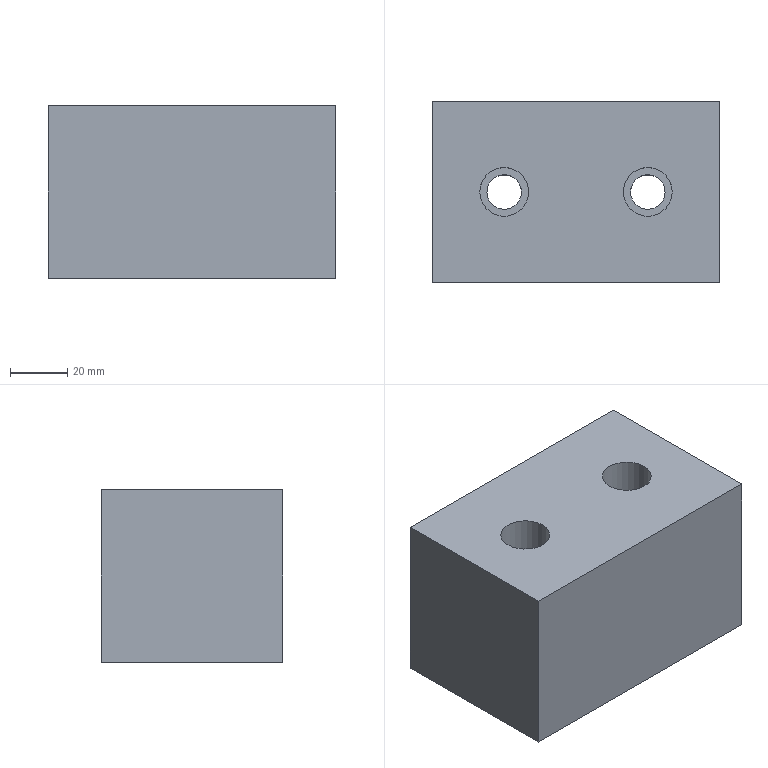Part | NX | features solid 2 | 1 solid | 12 faces | box 100 x 63 x 60 mm | volume 355318 mm3 | plane 8 | cylinder 4 | commonest cylinder face diameters 12 x2 17 x2
STEP:
#1=CARTESIAN_POINT('',(1065.,781.5,-55.));
#2=VERTEX_POINT('',#1);
#3=CARTESIAN_POINT('',(1065.,781.5,5.));
#4=VERTEX_POINT('',#3);
#5=CARTESIAN_POINT('',(1065.,781.5,-55.));
#6=DIRECTION('',(0.,0.,-1.));
#7=VECTOR('',#6,1000.);
#8=LINE('',#5,#7);
#9=EDGE_CURVE('',#2,#4,#8,.F.);
#10=ORIENTED_EDGE('',*,*,#9,.T.);
#11=CARTESIAN_POINT('',(1165.,781.5,5.));
#12=VERTEX_POINT('',#11);
#13=CARTESIAN_POINT('',(1065.,781.5,5.));
#14=DIRECTION('',(1.,0.,0.));
#15=VECTOR('',#14,1000.);
#16=LINE('',#13,#15);
#17=EDGE_CURVE('',#4,#12,#16,.T.);
#18=ORIENTED_EDGE('',*,*,#17,.T.);
#19=CARTESIAN_POINT('',(1165.,781.5,-55.));
#20=VERTEX_POINT('',#19);
#21=CARTESIAN_POINT('',(1165.,781.5,-55.));
#22=DIRECTION('',(0.,0.,1.));
#23=VECTOR('',#22,1000.);
#24=LINE('',#21,#23);
#25=EDGE_CURVE('',#20,#12,#24,.T.);
#26=ORIENTED_EDGE('',*,*,#25,.F.);
#27=CARTESIAN_POINT('',(1065.,781.5,-55.));
#28=DIRECTION('',(1.,0.,0.));
#29=VECTOR('',#28,1000.);
#30=LINE('',#27,#29);
#31=EDGE_CURVE('',#2,#20,#30,.T.);
#32=ORIENTED_EDGE('',*,*,#31,.F.);
#33=EDGE_LOOP('',(#10,#18,#26,#32));
#34=FACE_BOUND('',#33,.T.);
#35=CARTESIAN_POINT('',(1065.,781.5,-55.));
#36=DIRECTION('',(0.,1.,0.));
#37=DIRECTION('',(1.,0.,0.));
#38=AXIS2_PLACEMENT_3D('',#35,#36,#37);
#39=PLANE('',#38);
#40=ADVANCED_FACE('',(#34),#39,.T.);
#41=ORIENTED_EDGE('',*,*,#25,.T.);
#42=CARTESIAN_POINT('',(1165.,718.5,5.));
#43=VERTEX_POINT('',#42);
#44=CARTESIAN_POINT('',(1165.,780.,5.));
#45=DIRECTION('',(0.,-1.,0.));
#46=VECTOR('',#45,1000.);
#47=LINE('',#44,#46);
#48=EDGE_CURVE('',#12,#43,#47,.T.);
#49=ORIENTED_EDGE('',*,*,#48,.T.);
#50=CARTESIAN_POINT('',(1165.,718.5,-55.));
#51=VERTEX_POINT('',#50);
#52=CARTESIAN_POINT('',(1165.,718.5,-55.));
#53=DIRECTION('',(0.,0.,-1.));
#54=VECTOR('',#53,1000.);
#55=LINE('',#52,#54);
#56=EDGE_CURVE('',#51,#43,#55,.F.);
#57=ORIENTED_EDGE('',*,*,#56,.F.);
#58=CARTESIAN_POINT('',(1165.,780.,-55.));
#59=DIRECTION('',(0.,-1.,0.));
#60=VECTOR('',#59,1000.);
#61=LINE('',#58,#60);
#62=EDGE_CURVE('',#20,#51,#61,.T.);
#63=ORIENTED_EDGE('',*,*,#62,.F.);
#64=EDGE_LOOP('',(#41,#49,#57,#63));
#65=FACE_BOUND('',#64,.T.);
#66=CARTESIAN_POINT('',(1165.,780.,-55.));
#67=DIRECTION('',(1.,0.,0.));
#68=DIRECTION('',(0.,-1.,0.));
#69=AXIS2_PLACEMENT_3D('',#66,#67,#68);
#70=PLANE('',#69);
#71=ADVANCED_FACE('',(#65),#70,.T.);
#72=ORIENTED_EDGE('',*,*,#56,.T.);
#73=CARTESIAN_POINT('',(1065.,718.5,5.));
#74=VERTEX_POINT('',#73);
#75=CARTESIAN_POINT('',(1065.,718.5,5.));
#76=DIRECTION('',(-1.,0.,0.));
#77=VECTOR('',#76,1000.);
#78=LINE('',#75,#77);
#79=EDGE_CURVE('',#74,#43,#78,.F.);
#80=ORIENTED_EDGE('',*,*,#79,.F.);
#81=CARTESIAN_POINT('',(1065.,718.5,-55.));
#82=VERTEX_POINT('',#81);
#83=CARTESIAN_POINT('',(1065.,718.5,-55.));
#84=DIRECTION('',(0.,0.,1.));
#85=VECTOR('',#84,1000.);
#86=LINE('',#83,#85);
#87=EDGE_CURVE('',#82,#74,#86,.T.);
#88=ORIENTED_EDGE('',*,*,#87,.F.);
#89=CARTESIAN_POINT('',(1065.,718.5,-55.));
#90=DIRECTION('',(-1.,0.,0.));
#91=VECTOR('',#90,1000.);
#92=LINE('',#89,#91);
#93=EDGE_CURVE('',#82,#51,#92,.F.);
#94=ORIENTED_EDGE('',*,*,#93,.T.);
#95=EDGE_LOOP('',(#72,#80,#88,#94));
#96=FACE_BOUND('',#95,.T.);
#97=CARTESIAN_POINT('',(1065.,718.5,-55.));
#98=DIRECTION('',(0.,1.,0.));
#99=DIRECTION('',(1.,0.,0.));
#100=AXIS2_PLACEMENT_3D('',#97,#98,#99);
#101=PLANE('',#100);
#102=ADVANCED_FACE('',(#96),#101,.F.);
#103=CARTESIAN_POINT('',(1065.,780.,-55.));
#104=DIRECTION('',(0.,-1.,0.));
#105=VECTOR('',#104,1000.);
#106=LINE('',#103,#105);
#107=EDGE_CURVE('',#2,#82,#106,.T.);
#108=ORIENTED_EDGE('',*,*,#107,.T.);
#109=ORIENTED_EDGE('',*,*,#87,.T.);
#110=CARTESIAN_POINT('',(1065.,780.,5.));
#111=DIRECTION('',(0.,1.,0.));
#112=VECTOR('',#111,1000.);
#113=LINE('',#110,#112);
#114=EDGE_CURVE('',#4,#74,#113,.F.);
#115=ORIENTED_EDGE('',*,*,#114,.F.);
#116=ORIENTED_EDGE('',*,*,#9,.F.);
#117=EDGE_LOOP('',(#108,#109,#115,#116));
#118=FACE_BOUND('',#117,.T.);
#119=CARTESIAN_POINT('',(1065.,780.,-55.));
#120=DIRECTION('',(1.,0.,0.));
#121=DIRECTION('',(0.,-1.,0.));
#122=AXIS2_PLACEMENT_3D('',#119,#120,#121);
#123=PLANE('',#122);
#124=ADVANCED_FACE('',(#118),#123,.F.);
#125=CARTESIAN_POINT('',(1131.5,750.,5.));
#126=VERTEX_POINT('',#125);
#127=CARTESIAN_POINT('',(1140.,750.,5.));
#128=DIRECTION('',(0.,0.,1.));
#129=DIRECTION('',(-1.,0.,0.));
#130=AXIS2_PLACEMENT_3D('',#127,#128,#129);
#131=CIRCLE('',#130,8.5);
#132=EDGE_CURVE('',#126,#126,#131,.T.);
#133=ORIENTED_EDGE('',*,*,#132,.F.);
#134=EDGE_LOOP('',(#133));
#135=FACE_BOUND('',#134,.T.);
#136=CARTESIAN_POINT('',(1081.5,750.,5.));
#137=VERTEX_POINT('',#136);
#138=CARTESIAN_POINT('',(1090.,750.,5.));
#139=DIRECTION('',(0.,0.,1.));
#140=DIRECTION('',(-1.,0.,0.));
#141=AXIS2_PLACEMENT_3D('',#138,#139,#140);
#142=CIRCLE('',#141,8.5);
#143=EDGE_CURVE('',#137,#137,#142,.T.);
#144=ORIENTED_EDGE('',*,*,#143,.F.);
#145=EDGE_LOOP('',(#144));
#146=FACE_BOUND('',#145,.T.);
#147=ORIENTED_EDGE('',*,*,#79,.T.);
#148=ORIENTED_EDGE('',*,*,#48,.F.);
#149=ORIENTED_EDGE('',*,*,#17,.F.);
#150=ORIENTED_EDGE('',*,*,#114,.T.);
#151=EDGE_LOOP('',(#147,#148,#149,#150));
#152=FACE_BOUND('',#151,.T.);
#153=CARTESIAN_POINT('',(1065.,780.,5.));
#154=DIRECTION('',(0.,0.,1.));
#155=DIRECTION('',(1.,0.,0.));
#156=AXIS2_PLACEMENT_3D('',#153,#154,#155);
#157=PLANE('',#156);
#158=ADVANCED_FACE('',(#135,#146,#152),#157,.T.);
#159=CARTESIAN_POINT('',(1146.,750.,-55.));
#160=VERTEX_POINT('',#159);
#161=CARTESIAN_POINT('',(1140.,750.,-55.));
#162=DIRECTION('',(0.,0.,-1.));
#163=DIRECTION('',(1.,0.,0.));
#164=AXIS2_PLACEMENT_3D('',#161,#162,#163);
#165=CIRCLE('',#164,6.);
#166=EDGE_CURVE('',#160,#160,#165,.T.);
#167=ORIENTED_EDGE('',*,*,#166,.F.);
#168=EDGE_LOOP('',(#167));
#169=FACE_BOUND('',#168,.T.);
#170=CARTESIAN_POINT('',(1096.,750.,-55.));
#171=VERTEX_POINT('',#170);
#172=CARTESIAN_POINT('',(1090.,750.,-55.));
#173=DIRECTION('',(0.,0.,-1.));
#174=DIRECTION('',(1.,0.,0.));
#175=AXIS2_PLACEMENT_3D('',#172,#173,#174);
#176=CIRCLE('',#175,6.);
#177=EDGE_CURVE('',#171,#171,#176,.T.);
#178=ORIENTED_EDGE('',*,*,#177,.F.);
#179=EDGE_LOOP('',(#178));
#180=FACE_BOUND('',#179,.T.);
#181=ORIENTED_EDGE('',*,*,#93,.F.);
#182=ORIENTED_EDGE('',*,*,#107,.F.);
#183=ORIENTED_EDGE('',*,*,#31,.T.);
#184=ORIENTED_EDGE('',*,*,#62,.T.);
#185=EDGE_LOOP('',(#181,#182,#183,#184));
#186=FACE_BOUND('',#185,.T.);
#187=CARTESIAN_POINT('',(1065.,780.,-55.));
#188=DIRECTION('',(0.,0.,1.));
#189=DIRECTION('',(1.,0.,0.));
#190=AXIS2_PLACEMENT_3D('',#187,#188,#189);
#191=PLANE('',#190);
#192=ADVANCED_FACE('',(#169,#180,#186),#191,.F.);
#193=CARTESIAN_POINT('',(1084.,750.,-35.));
#194=VERTEX_POINT('',#193);
#195=CARTESIAN_POINT('',(1090.,750.,-35.));
#196=DIRECTION('',(0.,0.,1.));
#197=DIRECTION('',(-1.,0.,0.));
#198=AXIS2_PLACEMENT_3D('',#195,#196,#197);
#199=CIRCLE('',#198,6.);
#200=EDGE_CURVE('',#194,#194,#199,.T.);
#201=ORIENTED_EDGE('',*,*,#200,.F.);
#202=EDGE_LOOP('',(#201));
#203=FACE_BOUND('',#202,.T.);
#204=CARTESIAN_POINT('',(1081.5,750.,-35.));
#205=VERTEX_POINT('',#204);
#206=CARTESIAN_POINT('',(1090.,750.,-35.));
#207=DIRECTION('',(0.,0.,1.));
#208=DIRECTION('',(-1.,0.,0.));
#209=AXIS2_PLACEMENT_3D('',#206,#207,#208);
#210=CIRCLE('',#209,8.5);
#211=EDGE_CURVE('',#205,#205,#210,.T.);
#212=ORIENTED_EDGE('',*,*,#211,.T.);
#213=EDGE_LOOP('',(#212));
#214=FACE_BOUND('',#213,.T.);
#215=CARTESIAN_POINT('',(1090.,750.,-35.));
#216=DIRECTION('',(0.,0.,-1.));
#217=DIRECTION('',(-1.,0.,0.));
#218=AXIS2_PLACEMENT_3D('',#215,#216,#217);
#219=PLANE('',#218);
#220=ADVANCED_FACE('',(#203,#214),#219,.F.);
#221=ORIENTED_EDGE('',*,*,#211,.F.);
#222=EDGE_LOOP('',(#221));
#223=FACE_BOUND('',#222,.T.);
#224=ORIENTED_EDGE('',*,*,#143,.T.);
#225=EDGE_LOOP('',(#224));
#226=FACE_BOUND('',#225,.T.);
#227=CARTESIAN_POINT('',(1090.,750.,55.));
#228=DIRECTION('',(0.,0.,-1.));
#229=DIRECTION('',(-1.,0.,0.));
#230=AXIS2_PLACEMENT_3D('',#227,#228,#229);
#231=CYLINDRICAL_SURFACE('',#230,8.5);
#232=ADVANCED_FACE('',(#223,#226),#231,.F.);
#233=CARTESIAN_POINT('',(1134.,750.,-35.));
#234=VERTEX_POINT('',#233);
#235=CARTESIAN_POINT('',(1140.,750.,-35.));
#236=DIRECTION('',(0.,0.,1.));
#237=DIRECTION('',(-1.,0.,0.));
#238=AXIS2_PLACEMENT_3D('',#235,#236,#237);
#239=CIRCLE('',#238,6.);
#240=EDGE_CURVE('',#234,#234,#239,.T.);
#241=ORIENTED_EDGE('',*,*,#240,.F.);
#242=EDGE_LOOP('',(#241));
#243=FACE_BOUND('',#242,.T.);
#244=CARTESIAN_POINT('',(1131.5,750.,-35.));
#245=VERTEX_POINT('',#244);
#246=CARTESIAN_POINT('',(1140.,750.,-35.));
#247=DIRECTION('',(0.,0.,1.));
#248=DIRECTION('',(-1.,0.,0.));
#249=AXIS2_PLACEMENT_3D('',#246,#247,#248);
#250=CIRCLE('',#249,8.5);
#251=EDGE_CURVE('',#245,#245,#250,.T.);
#252=ORIENTED_EDGE('',*,*,#251,.T.);
#253=EDGE_LOOP('',(#252));
#254=FACE_BOUND('',#253,.T.);
#255=CARTESIAN_POINT('',(1140.,750.,-35.));
#256=DIRECTION('',(0.,0.,-1.));
#257=DIRECTION('',(-1.,0.,0.));
#258=AXIS2_PLACEMENT_3D('',#255,#256,#257);
#259=PLANE('',#258);
#260=ADVANCED_FACE('',(#243,#254),#259,.F.);
#261=ORIENTED_EDGE('',*,*,#251,.F.);
#262=EDGE_LOOP('',(#261));
#263=FACE_BOUND('',#262,.T.);
#264=ORIENTED_EDGE('',*,*,#132,.T.);
#265=EDGE_LOOP('',(#264));
#266=FACE_BOUND('',#265,.T.);
#267=CARTESIAN_POINT('',(1140.,750.,55.));
#268=DIRECTION('',(0.,0.,-1.));
#269=DIRECTION('',(-1.,0.,0.));
#270=AXIS2_PLACEMENT_3D('',#267,#268,#269);
#271=CYLINDRICAL_SURFACE('',#270,8.5);
#272=ADVANCED_FACE('',(#263,#266),#271,.F.);
#273=ORIENTED_EDGE('',*,*,#200,.T.);
#274=EDGE_LOOP('',(#273));
#275=FACE_BOUND('',#274,.T.);
#276=ORIENTED_EDGE('',*,*,#177,.T.);
#277=EDGE_LOOP('',(#276));
#278=FACE_BOUND('',#277,.T.);
#279=CARTESIAN_POINT('',(1090.,750.,-35.));
#280=DIRECTION('',(0.,0.,-1.));
#281=DIRECTION('',(-1.,0.,0.));
#282=AXIS2_PLACEMENT_3D('',#279,#280,#281);
#283=CYLINDRICAL_SURFACE('',#282,6.);
#284=ADVANCED_FACE('',(#275,#278),#283,.F.);
#285=ORIENTED_EDGE('',*,*,#240,.T.);
#286=EDGE_LOOP('',(#285));
#287=FACE_BOUND('',#286,.T.);
#288=ORIENTED_EDGE('',*,*,#166,.T.);
#289=EDGE_LOOP('',(#288));
#290=FACE_BOUND('',#289,.T.);
#291=CARTESIAN_POINT('',(1140.,750.,-35.));
#292=DIRECTION('',(0.,0.,-1.));
#293=DIRECTION('',(-1.,0.,0.));
#294=AXIS2_PLACEMENT_3D('',#291,#292,#293);
#295=CYLINDRICAL_SURFACE('',#294,6.);
#296=ADVANCED_FACE('',(#287,#290),#295,.F.);
#297=CLOSED_SHELL('',(#40,#71,#102,#124,#158,#192,#220,#232,#260,#272,#284,#296));
#298=MANIFOLD_SOLID_BREP('',#297);
#299=(LENGTH_UNIT()NAMED_UNIT(*)SI_UNIT(.MILLI.,.METRE.));
#300=UNCERTAINTY_MEASURE_WITH_UNIT(LENGTH_MEASURE(0.00001),#299,'','');
#301=(NAMED_UNIT(*)PLANE_ANGLE_UNIT()SI_UNIT($,.RADIAN.));
#302=(NAMED_UNIT(*)SI_UNIT($,.STERADIAN.)SOLID_ANGLE_UNIT());
#303=(GEOMETRIC_REPRESENTATION_CONTEXT(3)GLOBAL_UNCERTAINTY_ASSIGNED_CONTEXT((#300))GLOBAL_UNIT_ASSIGNED_CONTEXT((#299,#301,#302))REPRESENTATION_CONTEXT('',''));
#304=ADVANCED_BREP_SHAPE_REPRESENTATION('',(#298),#303);